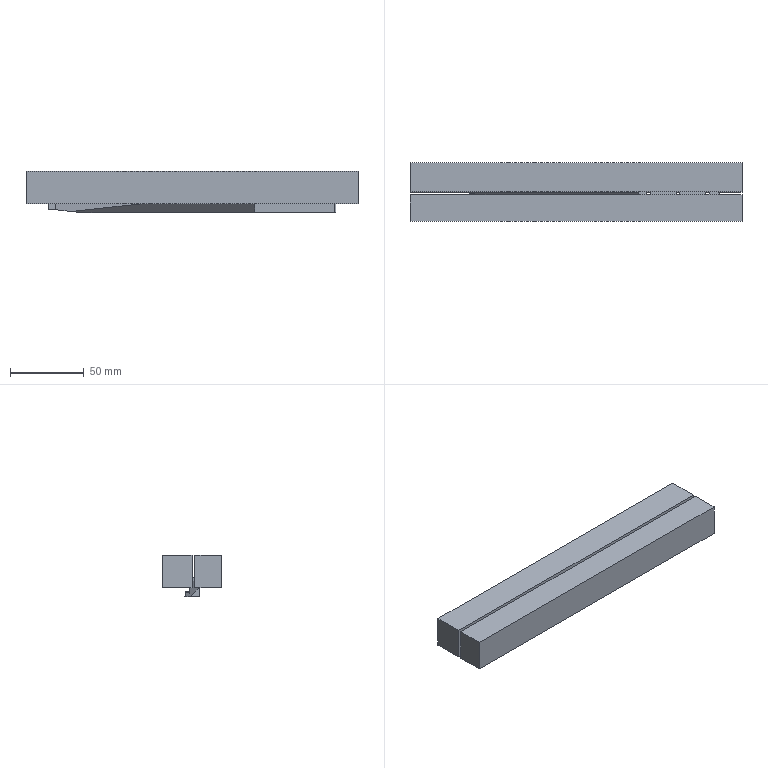Part | 3 solids | 82 faces | box 225.5 x 39.7 x 28 mm | volume 190881 mm3 | plane 61 | cylinder 21 | commonest cylinder face diameters 2 x10 1 x3 2.5 x3 8 x3 0.2 x2